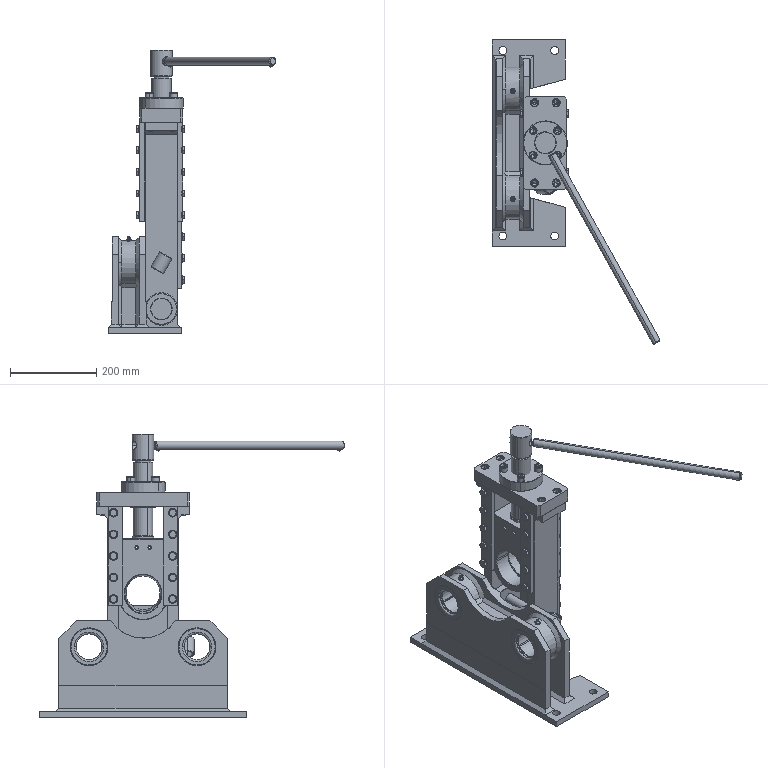Part | SolidWorks | 82 solids | 2017 faces | box 388.966 x 706.727 x 655.972 mm | volume 9412553 mm3 | plane 884 | cylinder 538 | cone 521 | spline 74 | commonest cylinder face diameters 10 x56 8.376 x52 10.5 x52 16 x52 20 x52 11 x40